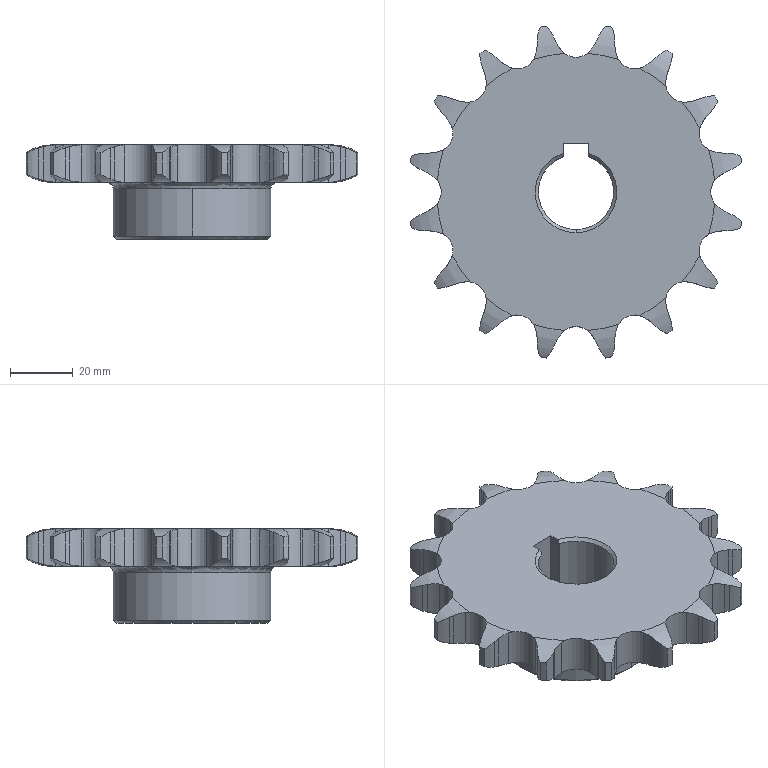Part | SolidWorks | features BaseBody 1 | 1 solid | 185 faces | box 105.504 x 105.504 x 30 mm | volume 102425 mm3 | cylinder 106 | plane 38 | spline 34 | cone 7 | commonest cylinder face diameters 19.857 x34 31.085 x32 12.029 x21 107.201 x16 50 x2 24 x1